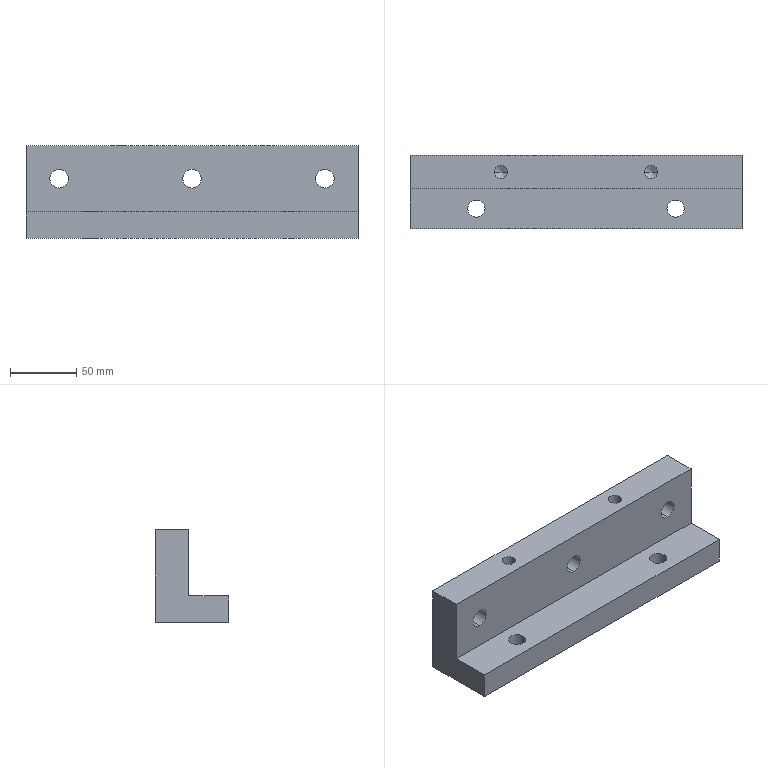Part | STEP file | CHAN DO | 1 solid | 26 faces | box 250 x 55 x 70 mm | volume 565670 mm3 | cylinder 14 | plane 8 | cone 4 | commonest cylinder face diameters 14 x6 10.106 x4 13 x4